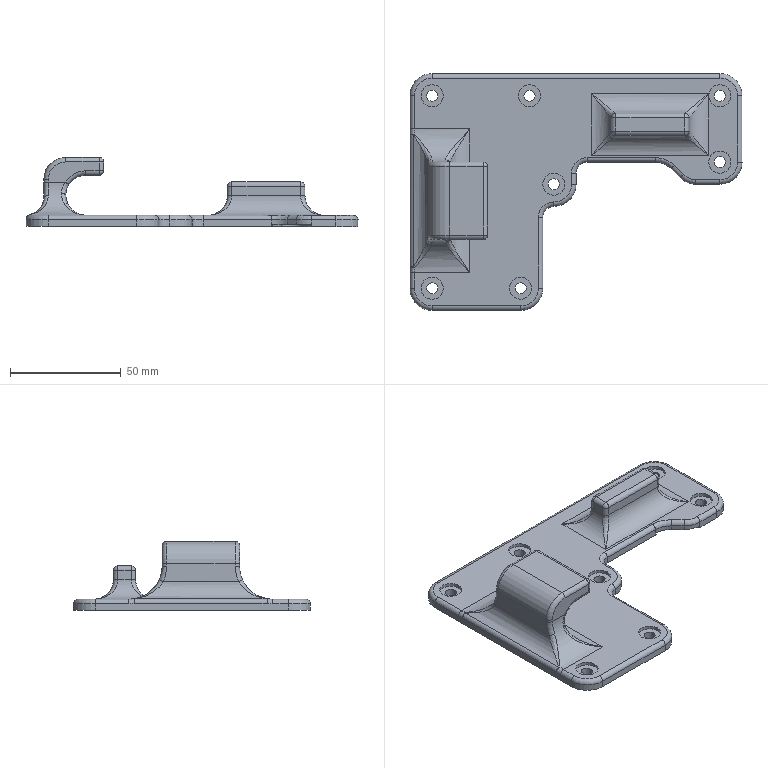Part | SolidWorks | features BaseBody 1 | 1 solid | 164 faces | box 150.004 x 107.006 x 31.21 mm | volume 73513 mm3 | cylinder 88 | plane 36 | torus 20 | spline 10 | sphere 10 | commonest cylinder face diameters 4 x31 10 x23 5 x14 20 x9 18 x6 6 x2